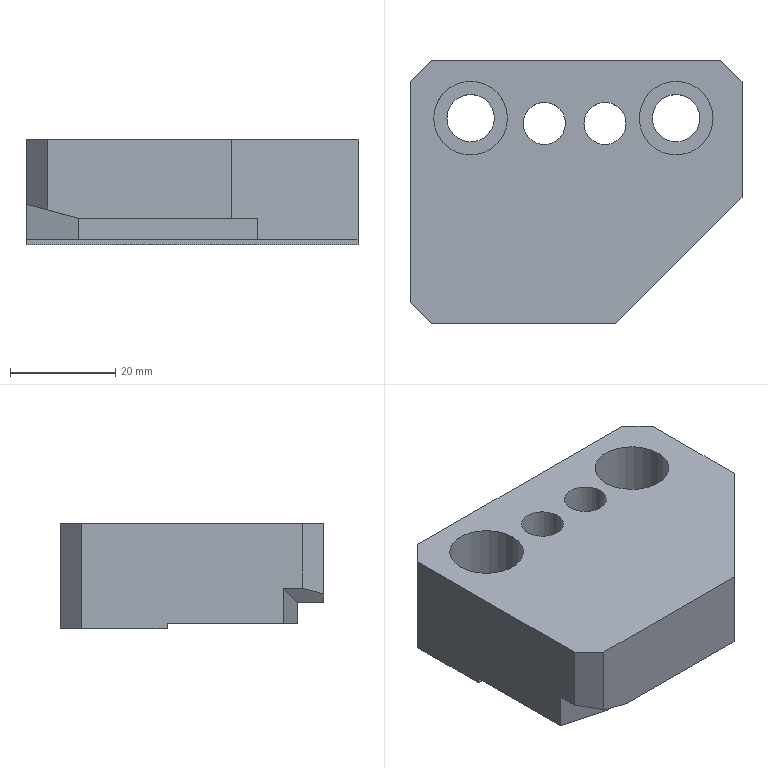Part | NX | features 20 2 | 1 solid | 24 faces | box 63 x 50 x 20 mm | volume 47897 mm3 | plane 18 | cylinder 6 | commonest cylinder face diameters 8.001 x2 9 x2 14 x2
STEP:
#1=CARTESIAN_POINT('',(190.002,447.223,-3.5));
#2=VERTEX_POINT('',#1);
#3=CARTESIAN_POINT('',(190.002,447.223,-2.5));
#4=VERTEX_POINT('',#3);
#5=CARTESIAN_POINT('',(190.002,447.223,11.5));
#6=DIRECTION('',(0.,0.,1.));
#7=VECTOR('',#6,1000.);
#8=LINE('',#5,#7);
#9=EDGE_CURVE('',#2,#4,#8,.T.);
#10=ORIENTED_EDGE('',*,*,#9,.F.);
#11=CARTESIAN_POINT('',(190.002,463.5,-3.5));
#12=VERTEX_POINT('',#11);
#13=CARTESIAN_POINT('',(190.002,450.5,-3.5));
#14=DIRECTION('',(0.,1.,0.));
#15=VECTOR('',#14,1000.);
#16=LINE('',#13,#15);
#17=EDGE_CURVE('',#2,#12,#16,.T.);
#18=ORIENTED_EDGE('',*,*,#17,.T.);
#19=CARTESIAN_POINT('',(190.002,463.5,16.5));
#20=VERTEX_POINT('',#19);
#21=CARTESIAN_POINT('',(190.002,463.5,11.5));
#22=DIRECTION('',(0.,0.,1.));
#23=VECTOR('',#22,1000.);
#24=LINE('',#21,#23);
#25=EDGE_CURVE('',#12,#20,#24,.T.);
#26=ORIENTED_EDGE('',*,*,#25,.T.);
#27=CARTESIAN_POINT('',(190.002,441.5,16.5));
#28=VERTEX_POINT('',#27);
#29=CARTESIAN_POINT('',(190.002,450.5,16.5));
#30=DIRECTION('',(0.,1.,0.));
#31=VECTOR('',#30,1000.);
#32=LINE('',#29,#31);
#33=EDGE_CURVE('',#28,#20,#32,.T.);
#34=ORIENTED_EDGE('',*,*,#33,.F.);
#35=CARTESIAN_POINT('',(190.002,441.5,-2.5));
#36=VERTEX_POINT('',#35);
#37=CARTESIAN_POINT('',(190.002,441.5,11.5));
#38=DIRECTION('',(0.,0.,-1.));
#39=VECTOR('',#38,1000.);
#40=LINE('',#37,#39);
#41=EDGE_CURVE('',#28,#36,#40,.T.);
#42=ORIENTED_EDGE('',*,*,#41,.T.);
#43=CARTESIAN_POINT('',(190.002,450.5,-2.5));
#44=DIRECTION('',(0.,1.,0.));
#45=VECTOR('',#44,1000.);
#46=LINE('',#43,#45);
#47=EDGE_CURVE('',#36,#4,#46,.T.);
#48=ORIENTED_EDGE('',*,*,#47,.T.);
#49=EDGE_LOOP('',(#10,#18,#26,#34,#42,#48));
#50=FACE_BOUND('',#49,.T.);
#51=CARTESIAN_POINT('',(190.002,450.5,11.5));
#52=DIRECTION('',(-1.,0.,0.));
#53=DIRECTION('',(0.,0.,-1.));
#54=AXIS2_PLACEMENT_3D('',#51,#52,#53);
#55=PLANE('',#54);
#56=ADVANCED_FACE('',(#50),#55,.F.);
#57=CARTESIAN_POINT('',(127.002,447.223,-2.5));
#58=VERTEX_POINT('',#57);
#59=CARTESIAN_POINT('',(127.002,447.223,-3.5));
#60=VERTEX_POINT('',#59);
#61=CARTESIAN_POINT('',(127.002,447.223,11.5));
#62=DIRECTION('',(0.,0.,-1.));
#63=VECTOR('',#62,1000.);
#64=LINE('',#61,#63);
#65=EDGE_CURVE('',#58,#60,#64,.T.);
#66=ORIENTED_EDGE('',*,*,#65,.F.);
#67=CARTESIAN_POINT('',(127.002,425.179,-2.5));
#68=VERTEX_POINT('',#67);
#69=CARTESIAN_POINT('',(127.002,417.5,-2.5));
#70=DIRECTION('',(0.,-1.,0.));
#71=VECTOR('',#70,1000.);
#72=LINE('',#69,#71);
#73=EDGE_CURVE('',#58,#68,#72,.T.);
#74=ORIENTED_EDGE('',*,*,#73,.T.);
#75=CARTESIAN_POINT('',(127.002,425.179,4.179));
#76=VERTEX_POINT('',#75);
#77=CARTESIAN_POINT('',(127.002,425.179,3.5));
#78=DIRECTION('',(0.,0.,1.));
#79=VECTOR('',#78,1000.);
#80=LINE('',#77,#79);
#81=EDGE_CURVE('',#68,#76,#80,.T.);
#82=ORIENTED_EDGE('',*,*,#81,.T.);
#83=CARTESIAN_POINT('',(127.002,421.5,4.179));
#84=VERTEX_POINT('',#83);
#85=CARTESIAN_POINT('',(127.002,425.179,4.179));
#86=DIRECTION('',(0.,-1.,0.));
#87=VECTOR('',#86,1000.);
#88=LINE('',#85,#87);
#89=EDGE_CURVE('',#76,#84,#88,.T.);
#90=ORIENTED_EDGE('',*,*,#89,.T.);
#91=CARTESIAN_POINT('',(127.002,421.5,16.5));
#92=VERTEX_POINT('',#91);
#93=CARTESIAN_POINT('',(127.002,421.5,11.5));
#94=DIRECTION('',(0.,0.,1.));
#95=VECTOR('',#94,1000.);
#96=LINE('',#93,#95);
#97=EDGE_CURVE('',#84,#92,#96,.T.);
#98=ORIENTED_EDGE('',*,*,#97,.T.);
#99=CARTESIAN_POINT('',(127.002,463.5,16.5));
#100=VERTEX_POINT('',#99);
#101=CARTESIAN_POINT('',(127.002,417.5,16.5));
#102=DIRECTION('',(0.,-1.,0.));
#103=VECTOR('',#102,1000.);
#104=LINE('',#101,#103);
#105=EDGE_CURVE('',#100,#92,#104,.T.);
#106=ORIENTED_EDGE('',*,*,#105,.F.);
#107=CARTESIAN_POINT('',(127.002,463.5,-3.5));
#108=VERTEX_POINT('',#107);
#109=CARTESIAN_POINT('',(127.002,463.5,11.5));
#110=DIRECTION('',(0.,0.,-1.));
#111=VECTOR('',#110,1000.);
#112=LINE('',#109,#111);
#113=EDGE_CURVE('',#100,#108,#112,.T.);
#114=ORIENTED_EDGE('',*,*,#113,.T.);
#115=CARTESIAN_POINT('',(127.002,417.5,-3.5));
#116=DIRECTION('',(0.,-1.,0.));
#117=VECTOR('',#116,1000.);
#118=LINE('',#115,#117);
#119=EDGE_CURVE('',#108,#60,#118,.T.);
#120=ORIENTED_EDGE('',*,*,#119,.T.);
#121=EDGE_LOOP('',(#66,#74,#82,#90,#98,#106,#114,#120));
#122=FACE_BOUND('',#121,.T.);
#123=CARTESIAN_POINT('',(127.002,417.5,11.5));
#124=DIRECTION('',(1.,0.,0.));
#125=DIRECTION('',(0.,0.,1.));
#126=AXIS2_PLACEMENT_3D('',#123,#124,#125);
#127=PLANE('',#126);
#128=ADVANCED_FACE('',(#122),#127,.F.);
#129=CARTESIAN_POINT('',(145.502,456.5,16.5));
#130=VERTEX_POINT('',#129);
#131=CARTESIAN_POINT('',(138.502,456.5,16.5));
#132=DIRECTION('',(0.,0.,1.));
#133=DIRECTION('',(1.,0.,0.));
#134=AXIS2_PLACEMENT_3D('',#131,#132,#133);
#135=CIRCLE('',#134,7.);
#136=EDGE_CURVE('',#130,#130,#135,.T.);
#137=ORIENTED_EDGE('',*,*,#136,.F.);
#138=EDGE_LOOP('',(#137));
#139=FACE_BOUND('',#138,.T.);
#140=CARTESIAN_POINT('',(184.502,456.5,16.5));
#141=VERTEX_POINT('',#140);
#142=CARTESIAN_POINT('',(177.502,456.5,16.5));
#143=DIRECTION('',(0.,0.,-1.));
#144=DIRECTION('',(1.,0.,0.));
#145=AXIS2_PLACEMENT_3D('',#142,#143,#144);
#146=CIRCLE('',#145,7.);
#147=EDGE_CURVE('',#141,#141,#146,.T.);
#148=ORIENTED_EDGE('',*,*,#147,.T.);
#149=EDGE_LOOP('',(#148));
#150=FACE_BOUND('',#149,.T.);
#151=ORIENTED_EDGE('',*,*,#105,.T.);
#152=CARTESIAN_POINT('',(131.002,417.5,16.5));
#153=VERTEX_POINT('',#152);
#154=CARTESIAN_POINT('',(127.002,421.5,16.5));
#155=DIRECTION('',(0.7071,-0.7071,0.));
#156=VECTOR('',#155,1000.);
#157=LINE('',#154,#156);
#158=EDGE_CURVE('',#92,#153,#157,.T.);
#159=ORIENTED_EDGE('',*,*,#158,.T.);
#160=CARTESIAN_POINT('',(166.002,417.5,16.5));
#161=VERTEX_POINT('',#160);
#162=CARTESIAN_POINT('',(104.002,417.5,16.5));
#163=DIRECTION('',(1.,0.,0.));
#164=VECTOR('',#163,1000.);
#165=LINE('',#162,#164);
#166=EDGE_CURVE('',#153,#161,#165,.T.);
#167=ORIENTED_EDGE('',*,*,#166,.T.);
#168=CARTESIAN_POINT('',(186.002,437.5,16.5));
#169=DIRECTION('',(0.7071,0.7071,0.));
#170=VECTOR('',#169,1000.);
#171=LINE('',#168,#170);
#172=EDGE_CURVE('',#161,#28,#171,.T.);
#173=ORIENTED_EDGE('',*,*,#172,.T.);
#174=ORIENTED_EDGE('',*,*,#33,.T.);
#175=CARTESIAN_POINT('',(186.002,467.5,16.5));
#176=VERTEX_POINT('',#175);
#177=CARTESIAN_POINT('',(190.002,463.5,16.5));
#178=DIRECTION('',(-0.7071,0.7071,0.));
#179=VECTOR('',#178,1000.);
#180=LINE('',#177,#179);
#181=EDGE_CURVE('',#20,#176,#180,.T.);
#182=ORIENTED_EDGE('',*,*,#181,.T.);
#183=CARTESIAN_POINT('',(131.002,467.5,16.5));
#184=VERTEX_POINT('',#183);
#185=CARTESIAN_POINT('',(24.002,467.5,16.5));
#186=DIRECTION('',(-1.,0.,0.));
#187=VECTOR('',#186,1000.);
#188=LINE('',#185,#187);
#189=EDGE_CURVE('',#176,#184,#188,.T.);
#190=ORIENTED_EDGE('',*,*,#189,.T.);
#191=CARTESIAN_POINT('',(131.002,467.5,16.5));
#192=DIRECTION('',(-0.7071,-0.7071,0.));
#193=VECTOR('',#192,1000.);
#194=LINE('',#191,#193);
#195=EDGE_CURVE('',#184,#100,#194,.T.);
#196=ORIENTED_EDGE('',*,*,#195,.T.);
#197=EDGE_LOOP('',(#151,#159,#167,#173,#174,#182,#190,#196));
#198=FACE_BOUND('',#197,.T.);
#199=CARTESIAN_POINT('',(156.502,455.5,16.5));
#200=VERTEX_POINT('',#199);
#201=CARTESIAN_POINT('',(152.502,455.5,16.5));
#202=DIRECTION('',(0.,0.,-1.));
#203=DIRECTION('',(1.,0.,0.));
#204=AXIS2_PLACEMENT_3D('',#201,#202,#203);
#205=CIRCLE('',#204,4.);
#206=EDGE_CURVE('',#200,#200,#205,.T.);
#207=ORIENTED_EDGE('',*,*,#206,.T.);
#208=EDGE_LOOP('',(#207));
#209=FACE_BOUND('',#208,.T.);
#210=CARTESIAN_POINT('',(168.002,455.5,16.5));
#211=VERTEX_POINT('',#210);
#212=CARTESIAN_POINT('',(164.002,455.5,16.5));
#213=DIRECTION('',(0.,0.,1.));
#214=DIRECTION('',(1.,0.,0.));
#215=AXIS2_PLACEMENT_3D('',#212,#213,#214);
#216=CIRCLE('',#215,4.);
#217=EDGE_CURVE('',#211,#211,#216,.T.);
#218=ORIENTED_EDGE('',*,*,#217,.F.);
#219=EDGE_LOOP('',(#218));
#220=FACE_BOUND('',#219,.T.);
#221=CARTESIAN_POINT('',(104.002,450.5,16.5));
#222=DIRECTION('',(0.,0.,1.));
#223=DIRECTION('',(-1.,0.,0.));
#224=AXIS2_PLACEMENT_3D('',#221,#222,#223);
#225=PLANE('',#224);
#226=ADVANCED_FACE('',(#139,#150,#198,#209,#220),#225,.T.);
#227=CARTESIAN_POINT('',(134.002,456.5,-3.5));
#228=VERTEX_POINT('',#227);
#229=CARTESIAN_POINT('',(138.502,456.5,-3.5));
#230=DIRECTION('',(0.,0.,1.));
#231=DIRECTION('',(-1.,0.,0.));
#232=AXIS2_PLACEMENT_3D('',#229,#230,#231);
#233=CIRCLE('',#232,4.5);
#234=EDGE_CURVE('',#228,#228,#233,.T.);
#235=ORIENTED_EDGE('',*,*,#234,.T.);
#236=EDGE_LOOP('',(#235));
#237=FACE_BOUND('',#236,.T.);
#238=CARTESIAN_POINT('',(182.002,456.5,-3.5));
#239=VERTEX_POINT('',#238);
#240=CARTESIAN_POINT('',(177.502,456.5,-3.5));
#241=DIRECTION('',(0.,0.,1.));
#242=DIRECTION('',(1.,0.,0.));
#243=AXIS2_PLACEMENT_3D('',#240,#241,#242);
#244=CIRCLE('',#243,4.5);
#245=EDGE_CURVE('',#239,#239,#244,.T.);
#246=ORIENTED_EDGE('',*,*,#245,.T.);
#247=EDGE_LOOP('',(#246));
#248=FACE_BOUND('',#247,.T.);
#249=CARTESIAN_POINT('',(156.502,455.5,-3.5));
#250=VERTEX_POINT('',#249);
#251=CARTESIAN_POINT('',(152.502,455.5,-3.5));
#252=DIRECTION('',(0.,0.,-1.));
#253=DIRECTION('',(1.,0.,0.));
#254=AXIS2_PLACEMENT_3D('',#251,#252,#253);
#255=CIRCLE('',#254,4.);
#256=EDGE_CURVE('',#250,#250,#255,.T.);
#257=ORIENTED_EDGE('',*,*,#256,.F.);
#258=EDGE_LOOP('',(#257));
#259=FACE_BOUND('',#258,.T.);
#260=CARTESIAN_POINT('',(168.002,455.5,-3.5));
#261=VERTEX_POINT('',#260);
#262=CARTESIAN_POINT('',(164.002,455.5,-3.5));
#263=DIRECTION('',(0.,0.,1.));
#264=DIRECTION('',(1.,0.,0.));
#265=AXIS2_PLACEMENT_3D('',#262,#263,#264);
#266=CIRCLE('',#265,4.);
#267=EDGE_CURVE('',#261,#261,#266,.T.);
#268=ORIENTED_EDGE('',*,*,#267,.T.);
#269=EDGE_LOOP('',(#268));
#270=FACE_BOUND('',#269,.T.);
#271=CARTESIAN_POINT('',(253.319,447.223,-3.5));
#272=DIRECTION('',(-1.,0.,0.));
#273=VECTOR('',#272,1000.);
#274=LINE('',#271,#273);
#275=EDGE_CURVE('',#2,#60,#274,.T.);
#276=ORIENTED_EDGE('',*,*,#275,.T.);
#277=ORIENTED_EDGE('',*,*,#119,.F.);
#278=CARTESIAN_POINT('',(131.002,467.5,-3.5));
#279=VERTEX_POINT('',#278);
#280=CARTESIAN_POINT('',(131.002,467.5,-3.5));
#281=DIRECTION('',(0.7071,0.7071,0.));
#282=VECTOR('',#281,1000.);
#283=LINE('',#280,#282);
#284=EDGE_CURVE('',#108,#279,#283,.T.);
#285=ORIENTED_EDGE('',*,*,#284,.T.);
#286=CARTESIAN_POINT('',(186.002,467.5,-3.5));
#287=VERTEX_POINT('',#286);
#288=CARTESIAN_POINT('',(24.002,467.5,-3.5));
#289=DIRECTION('',(-1.,0.,0.));
#290=VECTOR('',#289,1000.);
#291=LINE('',#288,#290);
#292=EDGE_CURVE('',#287,#279,#291,.T.);
#293=ORIENTED_EDGE('',*,*,#292,.F.);
#294=CARTESIAN_POINT('',(190.002,463.5,-3.5));
#295=DIRECTION('',(0.7071,-0.7071,0.));
#296=VECTOR('',#295,1000.);
#297=LINE('',#294,#296);
#298=EDGE_CURVE('',#287,#12,#297,.T.);
#299=ORIENTED_EDGE('',*,*,#298,.T.);
#300=ORIENTED_EDGE('',*,*,#17,.F.);
#301=EDGE_LOOP('',(#276,#277,#285,#293,#299,#300));
#302=FACE_BOUND('',#301,.T.);
#303=CARTESIAN_POINT('',(104.002,450.5,-3.5));
#304=DIRECTION('',(0.,0.,1.));
#305=DIRECTION('',(-1.,0.,0.));
#306=AXIS2_PLACEMENT_3D('',#303,#304,#305);
#307=PLANE('',#306);
#308=ADVANCED_FACE('',(#237,#248,#259,#270,#302),#307,.F.);
#309=ORIENTED_EDGE('',*,*,#206,.F.);
#310=EDGE_LOOP('',(#309));
#311=FACE_BOUND('',#310,.T.);
#312=ORIENTED_EDGE('',*,*,#256,.T.);
#313=EDGE_LOOP('',(#312));
#314=FACE_BOUND('',#313,.T.);
#315=CARTESIAN_POINT('',(152.502,455.5,42.5));
#316=DIRECTION('',(0.,0.,-1.));
#317=DIRECTION('',(1.,0.,0.));
#318=AXIS2_PLACEMENT_3D('',#315,#316,#317);
#319=CYLINDRICAL_SURFACE('',#318,4.);
#320=ADVANCED_FACE('',(#311,#314),#319,.F.);
#321=ORIENTED_EDGE('',*,*,#217,.T.);
#322=EDGE_LOOP('',(#321));
#323=FACE_BOUND('',#322,.T.);
#324=ORIENTED_EDGE('',*,*,#267,.F.);
#325=EDGE_LOOP('',(#324));
#326=FACE_BOUND('',#325,.T.);
#327=CARTESIAN_POINT('',(164.002,455.5,42.5));
#328=DIRECTION('',(0.,0.,-1.));
#329=DIRECTION('',(1.,0.,0.));
#330=AXIS2_PLACEMENT_3D('',#327,#328,#329);
#331=CYLINDRICAL_SURFACE('',#330,4.);
#332=ADVANCED_FACE('',(#323,#326),#331,.F.);
#333=ORIENTED_EDGE('',*,*,#136,.T.);
#334=EDGE_LOOP('',(#333));
#335=FACE_BOUND('',#334,.T.);
#336=CARTESIAN_POINT('',(145.502,456.5,6.5));
#337=VERTEX_POINT('',#336);
#338=CARTESIAN_POINT('',(138.502,456.5,6.5));
#339=DIRECTION('',(0.,0.,1.));
#340=DIRECTION('',(1.,0.,0.));
#341=AXIS2_PLACEMENT_3D('',#338,#339,#340);
#342=CIRCLE('',#341,7.);
#343=EDGE_CURVE('',#337,#337,#342,.T.);
#344=ORIENTED_EDGE('',*,*,#343,.F.);
#345=EDGE_LOOP('',(#344));
#346=FACE_BOUND('',#345,.T.);
#347=CARTESIAN_POINT('',(138.502,456.5,11.5));
#348=DIRECTION('',(0.,0.,-1.));
#349=DIRECTION('',(-1.,0.,0.));
#350=AXIS2_PLACEMENT_3D('',#347,#348,#349);
#351=CYLINDRICAL_SURFACE('',#350,7.);
#352=ADVANCED_FACE('',(#335,#346),#351,.F.);
#353=ORIENTED_EDGE('',*,*,#147,.F.);
#354=EDGE_LOOP('',(#353));
#355=FACE_BOUND('',#354,.T.);
#356=CARTESIAN_POINT('',(184.502,456.5,6.5));
#357=VERTEX_POINT('',#356);
#358=CARTESIAN_POINT('',(177.502,456.5,6.5));
#359=DIRECTION('',(0.,0.,1.));
#360=DIRECTION('',(1.,0.,0.));
#361=AXIS2_PLACEMENT_3D('',#358,#359,#360);
#362=CIRCLE('',#361,7.);
#363=EDGE_CURVE('',#357,#357,#362,.T.);
#364=ORIENTED_EDGE('',*,*,#363,.F.);
#365=EDGE_LOOP('',(#364));
#366=FACE_BOUND('',#365,.T.);
#367=CARTESIAN_POINT('',(177.502,456.5,11.5));
#368=DIRECTION('',(0.,0.,-1.));
#369=DIRECTION('',(-1.,0.,0.));
#370=AXIS2_PLACEMENT_3D('',#367,#368,#369);
#371=CYLINDRICAL_SURFACE('',#370,7.);
#372=ADVANCED_FACE('',(#355,#366),#371,.F.);
#373=ORIENTED_EDGE('',*,*,#25,.F.);
#374=ORIENTED_EDGE('',*,*,#298,.F.);
#375=CARTESIAN_POINT('',(186.002,467.5,11.5));
#376=DIRECTION('',(0.,0.,-1.));
#377=VECTOR('',#376,1000.);
#378=LINE('',#375,#377);
#379=EDGE_CURVE('',#176,#287,#378,.T.);
#380=ORIENTED_EDGE('',*,*,#379,.F.);
#381=ORIENTED_EDGE('',*,*,#181,.F.);
#382=EDGE_LOOP('',(#373,#374,#380,#381));
#383=FACE_BOUND('',#382,.T.);
#384=CARTESIAN_POINT('',(190.002,463.5,11.5));
#385=DIRECTION('',(-0.7071,-0.7071,0.));
#386=DIRECTION('',(0.,0.,-1.));
#387=AXIS2_PLACEMENT_3D('',#384,#385,#386);
#388=PLANE('',#387);
#389=ADVANCED_FACE('',(#383),#388,.F.);
#390=ORIENTED_EDGE('',*,*,#379,.T.);
#391=ORIENTED_EDGE('',*,*,#292,.T.);
#392=CARTESIAN_POINT('',(131.002,467.5,11.5));
#393=DIRECTION('',(0.,0.,1.));
#394=VECTOR('',#393,1000.);
#395=LINE('',#392,#394);
#396=EDGE_CURVE('',#279,#184,#395,.T.);
#397=ORIENTED_EDGE('',*,*,#396,.T.);
#398=ORIENTED_EDGE('',*,*,#189,.F.);
#399=EDGE_LOOP('',(#390,#391,#397,#398));
#400=FACE_BOUND('',#399,.T.);
#401=CARTESIAN_POINT('',(24.002,467.5,11.5));
#402=DIRECTION('',(0.,-1.,0.));
#403=DIRECTION('',(0.,0.,-1.));
#404=AXIS2_PLACEMENT_3D('',#401,#402,#403);
#405=PLANE('',#404);
#406=ADVANCED_FACE('',(#400),#405,.F.);
#407=ORIENTED_EDGE('',*,*,#396,.F.);
#408=ORIENTED_EDGE('',*,*,#284,.F.);
#409=ORIENTED_EDGE('',*,*,#113,.F.);
#410=ORIENTED_EDGE('',*,*,#195,.F.);
#411=EDGE_LOOP('',(#407,#408,#409,#410));
#412=FACE_BOUND('',#411,.T.);
#413=CARTESIAN_POINT('',(131.002,467.5,11.5));
#414=DIRECTION('',(0.7071,-0.7071,0.));
#415=DIRECTION('',(0.,0.,-1.));
#416=AXIS2_PLACEMENT_3D('',#413,#414,#415);
#417=PLANE('',#416);
#418=ADVANCED_FACE('',(#412),#417,.F.);
#419=CARTESIAN_POINT('',(143.002,456.5,6.5));
#420=VERTEX_POINT('',#419);
#421=CARTESIAN_POINT('',(138.502,456.5,6.5));
#422=DIRECTION('',(0.,0.,1.));
#423=DIRECTION('',(1.,0.,0.));
#424=AXIS2_PLACEMENT_3D('',#421,#422,#423);
#425=CIRCLE('',#424,4.5);
#426=EDGE_CURVE('',#420,#420,#425,.T.);
#427=ORIENTED_EDGE('',*,*,#426,.F.);
#428=EDGE_LOOP('',(#427));
#429=FACE_BOUND('',#428,.T.);
#430=ORIENTED_EDGE('',*,*,#343,.T.);
#431=EDGE_LOOP('',(#430));
#432=FACE_BOUND('',#431,.T.);
#433=CARTESIAN_POINT('',(278.002,322.3,6.5));
#434=DIRECTION('',(0.,0.,1.));
#435=DIRECTION('',(0.,1.,0.));
#436=AXIS2_PLACEMENT_3D('',#433,#434,#435);
#437=PLANE('',#436);
#438=ADVANCED_FACE('',(#429,#432),#437,.T.);
#439=ORIENTED_EDGE('',*,*,#426,.T.);
#440=EDGE_LOOP('',(#439));
#441=FACE_BOUND('',#440,.T.);
#442=ORIENTED_EDGE('',*,*,#234,.F.);
#443=EDGE_LOOP('',(#442));
#444=FACE_BOUND('',#443,.T.);
#445=CARTESIAN_POINT('',(138.502,456.5,-18.5));
#446=DIRECTION('',(0.,0.,-1.));
#447=DIRECTION('',(-1.,0.,0.));
#448=AXIS2_PLACEMENT_3D('',#445,#446,#447);
#449=CYLINDRICAL_SURFACE('',#448,4.5);
#450=ADVANCED_FACE('',(#441,#444),#449,.F.);
#451=CARTESIAN_POINT('',(182.002,456.5,6.5));
#452=VERTEX_POINT('',#451);
#453=CARTESIAN_POINT('',(177.502,456.5,6.5));
#454=DIRECTION('',(0.,0.,1.));
#455=DIRECTION('',(1.,0.,0.));
#456=AXIS2_PLACEMENT_3D('',#453,#454,#455);
#457=CIRCLE('',#456,4.5);
#458=EDGE_CURVE('',#452,#452,#457,.T.);
#459=ORIENTED_EDGE('',*,*,#458,.F.);
#460=EDGE_LOOP('',(#459));
#461=FACE_BOUND('',#460,.T.);
#462=ORIENTED_EDGE('',*,*,#363,.T.);
#463=EDGE_LOOP('',(#462));
#464=FACE_BOUND('',#463,.T.);
#465=CARTESIAN_POINT('',(317.002,322.3,6.5));
#466=DIRECTION('',(0.,0.,1.));
#467=DIRECTION('',(0.,1.,0.));
#468=AXIS2_PLACEMENT_3D('',#465,#466,#467);
#469=PLANE('',#468);
#470=ADVANCED_FACE('',(#461,#464),#469,.T.);
#471=ORIENTED_EDGE('',*,*,#458,.T.);
#472=EDGE_LOOP('',(#471));
#473=FACE_BOUND('',#472,.T.);
#474=ORIENTED_EDGE('',*,*,#245,.F.);
#475=EDGE_LOOP('',(#474));
#476=FACE_BOUND('',#475,.T.);
#477=CARTESIAN_POINT('',(177.502,456.5,-18.5));
#478=DIRECTION('',(0.,0.,-1.));
#479=DIRECTION('',(-1.,0.,0.));
#480=AXIS2_PLACEMENT_3D('',#477,#478,#479);
#481=CYLINDRICAL_SURFACE('',#480,4.5);
#482=ADVANCED_FACE('',(#473,#476),#481,.F.);
#483=CARTESIAN_POINT('',(104.002,447.223,-2.5));
#484=DIRECTION('',(1.,0.,0.));
#485=VECTOR('',#484,1000.);
#486=LINE('',#483,#485);
#487=EDGE_CURVE('',#58,#4,#486,.T.);
#488=ORIENTED_EDGE('',*,*,#487,.F.);
#489=ORIENTED_EDGE('',*,*,#65,.T.);
#490=ORIENTED_EDGE('',*,*,#275,.F.);
#491=ORIENTED_EDGE('',*,*,#9,.T.);
#492=EDGE_LOOP('',(#488,#489,#490,#491));
#493=FACE_BOUND('',#492,.T.);
#494=CARTESIAN_POINT('',(253.319,447.223,-21.));
#495=DIRECTION('',(0.,-1.,0.));
#496=DIRECTION('',(0.,0.,1.));
#497=AXIS2_PLACEMENT_3D('',#494,#495,#496);
#498=PLANE('',#497);
#499=ADVANCED_FACE('',(#493),#498,.T.);
#500=CARTESIAN_POINT('',(171.002,422.5,1.5));
#501=VERTEX_POINT('',#500);
#502=CARTESIAN_POINT('',(137.002,422.5,1.5));
#503=VERTEX_POINT('',#502);
#504=CARTESIAN_POINT('',(94.,422.5,1.5));
#505=DIRECTION('',(-1.,0.,0.));
#506=VECTOR('',#505,1000.);
#507=LINE('',#504,#506);
#508=EDGE_CURVE('',#501,#503,#507,.T.);
#509=ORIENTED_EDGE('',*,*,#508,.F.);
#510=CARTESIAN_POINT('',(166.002,417.5,1.5));
#511=VERTEX_POINT('',#510);
#512=CARTESIAN_POINT('',(186.002,437.5,1.5));
#513=DIRECTION('',(-0.7071,-0.7071,0.));
#514=VECTOR('',#513,1000.);
#515=LINE('',#512,#514);
#516=EDGE_CURVE('',#501,#511,#515,.T.);
#517=ORIENTED_EDGE('',*,*,#516,.T.);
#518=CARTESIAN_POINT('',(137.002,417.5,1.5));
#519=VERTEX_POINT('',#518);
#520=CARTESIAN_POINT('',(104.002,417.5,1.5));
#521=DIRECTION('',(-1.,0.,0.));
#522=VECTOR('',#521,1000.);
#523=LINE('',#520,#522);
#524=EDGE_CURVE('',#511,#519,#523,.T.);
#525=ORIENTED_EDGE('',*,*,#524,.T.);
#526=CARTESIAN_POINT('',(137.002,417.5,1.5));
#527=DIRECTION('',(0.,1.,0.));
#528=VECTOR('',#527,1000.);
#529=LINE('',#526,#528);
#530=EDGE_CURVE('',#519,#503,#529,.T.);
#531=ORIENTED_EDGE('',*,*,#530,.T.);
#532=EDGE_LOOP('',(#509,#517,#525,#531));
#533=FACE_BOUND('',#532,.T.);
#534=CARTESIAN_POINT('',(126.272,396.891,1.5));
#535=DIRECTION('',(0.,0.,-1.));
#536=DIRECTION('',(1.,0.,0.));
#537=AXIS2_PLACEMENT_3D('',#534,#535,#536);
#538=PLANE('',#537);
#539=ADVANCED_FACE('',(#533),#538,.T.);
#540=CARTESIAN_POINT('',(137.001,422.5,1.5));
#541=VERTEX_POINT('',#540);
#542=CARTESIAN_POINT('',(137.001,422.5,1.5));
#543=DIRECTION('',(-0.9351,0.2506,0.2506));
#544=VECTOR('',#543,1000.);
#545=LINE('',#542,#544);
#546=EDGE_CURVE('',#541,#76,#545,.T.);
#547=ORIENTED_EDGE('',*,*,#546,.F.);
#548=CARTESIAN_POINT('',(192.981,422.5,-13.5));
#549=DIRECTION('',(-0.9659,0.,0.2588));
#550=VECTOR('',#549,1000.);
#551=LINE('',#548,#550);
#552=EDGE_CURVE('',#503,#541,#551,.T.);
#553=ORIENTED_EDGE('',*,*,#552,.F.);
#554=ORIENTED_EDGE('',*,*,#530,.F.);
#555=CARTESIAN_POINT('',(131.002,417.5,3.108));
#556=VERTEX_POINT('',#555);
#557=CARTESIAN_POINT('',(137.002,417.5,1.5));
#558=DIRECTION('',(0.9659,0.,-0.2588));
#559=VECTOR('',#558,1000.);
#560=LINE('',#557,#559);
#561=EDGE_CURVE('',#556,#519,#560,.T.);
#562=ORIENTED_EDGE('',*,*,#561,.F.);
#563=CARTESIAN_POINT('',(144.053,404.449,-0.3894));
#564=DIRECTION('',(-0.6947,0.6947,0.1862));
#565=VECTOR('',#564,1000.);
#566=LINE('',#563,#565);
#567=EDGE_CURVE('',#556,#84,#566,.T.);
#568=ORIENTED_EDGE('',*,*,#567,.T.);
#569=ORIENTED_EDGE('',*,*,#89,.F.);
#570=EDGE_LOOP('',(#547,#553,#554,#562,#568,#569));
#571=FACE_BOUND('',#570,.T.);
#572=CARTESIAN_POINT('',(137.002,396.891,1.5));
#573=DIRECTION('',(-0.2588,0.,-0.9659));
#574=DIRECTION('',(0.9659,0.,-0.2588));
#575=AXIS2_PLACEMENT_3D('',#572,#573,#574);
#576=PLANE('',#575);
#577=ADVANCED_FACE('',(#571),#576,.T.);
#578=CARTESIAN_POINT('',(131.002,417.5,11.5));
#579=DIRECTION('',(0.,0.,-1.));
#580=VECTOR('',#579,1000.);
#581=LINE('',#578,#580);
#582=EDGE_CURVE('',#153,#556,#581,.T.);
#583=ORIENTED_EDGE('',*,*,#582,.T.);
#584=ORIENTED_EDGE('',*,*,#561,.T.);
#585=ORIENTED_EDGE('',*,*,#524,.F.);
#586=CARTESIAN_POINT('',(166.002,417.5,11.5));
#587=DIRECTION('',(0.,0.,1.));
#588=VECTOR('',#587,1000.);
#589=LINE('',#586,#588);
#590=EDGE_CURVE('',#511,#161,#589,.T.);
#591=ORIENTED_EDGE('',*,*,#590,.T.);
#592=ORIENTED_EDGE('',*,*,#166,.F.);
#593=EDGE_LOOP('',(#583,#584,#585,#591,#592));
#594=FACE_BOUND('',#593,.T.);
#595=CARTESIAN_POINT('',(104.002,417.5,11.5));
#596=DIRECTION('',(0.,1.,0.));
#597=DIRECTION('',(0.,0.,1.));
#598=AXIS2_PLACEMENT_3D('',#595,#596,#597);
#599=PLANE('',#598);
#600=ADVANCED_FACE('',(#594),#599,.F.);
#601=ORIENTED_EDGE('',*,*,#97,.F.);
#602=ORIENTED_EDGE('',*,*,#567,.F.);
#603=ORIENTED_EDGE('',*,*,#582,.F.);
#604=ORIENTED_EDGE('',*,*,#158,.F.);
#605=EDGE_LOOP('',(#601,#602,#603,#604));
#606=FACE_BOUND('',#605,.T.);
#607=CARTESIAN_POINT('',(127.002,421.5,11.5));
#608=DIRECTION('',(0.7071,0.7071,0.));
#609=DIRECTION('',(0.,0.,-1.));
#610=AXIS2_PLACEMENT_3D('',#607,#608,#609);
#611=PLANE('',#610);
#612=ADVANCED_FACE('',(#606),#611,.F.);
#613=CARTESIAN_POINT('',(137.001,422.5,-2.5));
#614=VERTEX_POINT('',#613);
#615=CARTESIAN_POINT('',(137.001,422.5,-2.5));
#616=DIRECTION('',(0.9659,-0.2588,0.));
#617=VECTOR('',#616,1000.);
#618=LINE('',#615,#617);
#619=EDGE_CURVE('',#68,#614,#618,.T.);
#620=ORIENTED_EDGE('',*,*,#619,.T.);
#621=CARTESIAN_POINT('',(137.001,422.5,3.5));
#622=DIRECTION('',(0.,0.,-1.));
#623=VECTOR('',#622,1000.);
#624=LINE('',#621,#623);
#625=EDGE_CURVE('',#541,#614,#624,.T.);
#626=ORIENTED_EDGE('',*,*,#625,.F.);
#627=ORIENTED_EDGE('',*,*,#546,.T.);
#628=ORIENTED_EDGE('',*,*,#81,.F.);
#629=EDGE_LOOP('',(#620,#626,#627,#628));
#630=FACE_BOUND('',#629,.T.);
#631=CARTESIAN_POINT('',(137.001,422.5,3.5));
#632=DIRECTION('',(0.2588,0.9659,0.));
#633=DIRECTION('',(0.9659,-0.2588,0.));
#634=AXIS2_PLACEMENT_3D('',#631,#632,#633);
#635=PLANE('',#634);
#636=ADVANCED_FACE('',(#630),#635,.F.);
#637=CARTESIAN_POINT('',(171.002,422.5,-2.5));
#638=VERTEX_POINT('',#637);
#639=CARTESIAN_POINT('',(94.,422.5,-2.5));
#640=DIRECTION('',(1.,0.,0.));
#641=VECTOR('',#640,1000.);
#642=LINE('',#639,#641);
#643=EDGE_CURVE('',#614,#638,#642,.T.);
#644=ORIENTED_EDGE('',*,*,#643,.T.);
#645=CARTESIAN_POINT('',(171.002,422.5,11.5));
#646=DIRECTION('',(0.,0.,-1.));
#647=VECTOR('',#646,1000.);
#648=LINE('',#645,#647);
#649=EDGE_CURVE('',#501,#638,#648,.T.);
#650=ORIENTED_EDGE('',*,*,#649,.F.);
#651=ORIENTED_EDGE('',*,*,#508,.T.);
#652=ORIENTED_EDGE('',*,*,#552,.T.);
#653=ORIENTED_EDGE('',*,*,#625,.T.);
#654=EDGE_LOOP('',(#644,#650,#651,#652,#653));
#655=FACE_BOUND('',#654,.T.);
#656=CARTESIAN_POINT('',(94.,422.5,3.5));
#657=DIRECTION('',(0.,1.,0.));
#658=DIRECTION('',(0.,0.,1.));
#659=AXIS2_PLACEMENT_3D('',#656,#657,#658);
#660=PLANE('',#659);
#661=ADVANCED_FACE('',(#655),#660,.F.);
#662=ORIENTED_EDGE('',*,*,#41,.F.);
#663=ORIENTED_EDGE('',*,*,#172,.F.);
#664=ORIENTED_EDGE('',*,*,#590,.F.);
#665=ORIENTED_EDGE('',*,*,#516,.F.);
#666=ORIENTED_EDGE('',*,*,#649,.T.);
#667=CARTESIAN_POINT('',(151.502,403.,-2.5));
#668=DIRECTION('',(-0.7071,-0.7071,0.));
#669=VECTOR('',#668,1000.);
#670=LINE('',#667,#669);
#671=EDGE_CURVE('',#36,#638,#670,.T.);
#672=ORIENTED_EDGE('',*,*,#671,.F.);
#673=EDGE_LOOP('',(#662,#663,#664,#665,#666,#672));
#674=FACE_BOUND('',#673,.T.);
#675=CARTESIAN_POINT('',(186.002,437.5,11.5));
#676=DIRECTION('',(-0.7071,0.7071,0.));
#677=DIRECTION('',(0.,0.,-1.));
#678=AXIS2_PLACEMENT_3D('',#675,#676,#677);
#679=PLANE('',#678);
#680=ADVANCED_FACE('',(#674),#679,.F.);
#681=ORIENTED_EDGE('',*,*,#73,.F.);
#682=ORIENTED_EDGE('',*,*,#487,.T.);
#683=ORIENTED_EDGE('',*,*,#47,.F.);
#684=ORIENTED_EDGE('',*,*,#671,.T.);
#685=ORIENTED_EDGE('',*,*,#643,.F.);
#686=ORIENTED_EDGE('',*,*,#619,.F.);
#687=EDGE_LOOP('',(#681,#682,#683,#684,#685,#686));
#688=FACE_BOUND('',#687,.T.);
#689=CARTESIAN_POINT('',(104.002,450.5,-2.5));
#690=DIRECTION('',(0.,0.,1.));
#691=DIRECTION('',(-1.,0.,0.));
#692=AXIS2_PLACEMENT_3D('',#689,#690,#691);
#693=PLANE('',#692);
#694=ADVANCED_FACE('',(#688),#693,.F.);
#695=CLOSED_SHELL('',(#56,#128,#226,#308,#320,#332,#352,#372,#389,#406,#418,#438,#450,#470,#482,#499,#539,#577,#600,#612,#636,#661,#680,#694));
#696=MANIFOLD_SOLID_BREP('',#695);
#697=(LENGTH_UNIT()NAMED_UNIT(*)SI_UNIT(.MILLI.,.METRE.));
#698=UNCERTAINTY_MEASURE_WITH_UNIT(LENGTH_MEASURE(0.00001),#697,'','');
#699=(NAMED_UNIT(*)PLANE_ANGLE_UNIT()SI_UNIT($,.RADIAN.));
#700=(NAMED_UNIT(*)SI_UNIT($,.STERADIAN.)SOLID_ANGLE_UNIT());
#701=(GEOMETRIC_REPRESENTATION_CONTEXT(3)GLOBAL_UNCERTAINTY_ASSIGNED_CONTEXT((#698))GLOBAL_UNIT_ASSIGNED_CONTEXT((#697,#699,#700))REPRESENTATION_CONTEXT('',''));
#702=ADVANCED_BREP_SHAPE_REPRESENTATION('',(#696),#701);